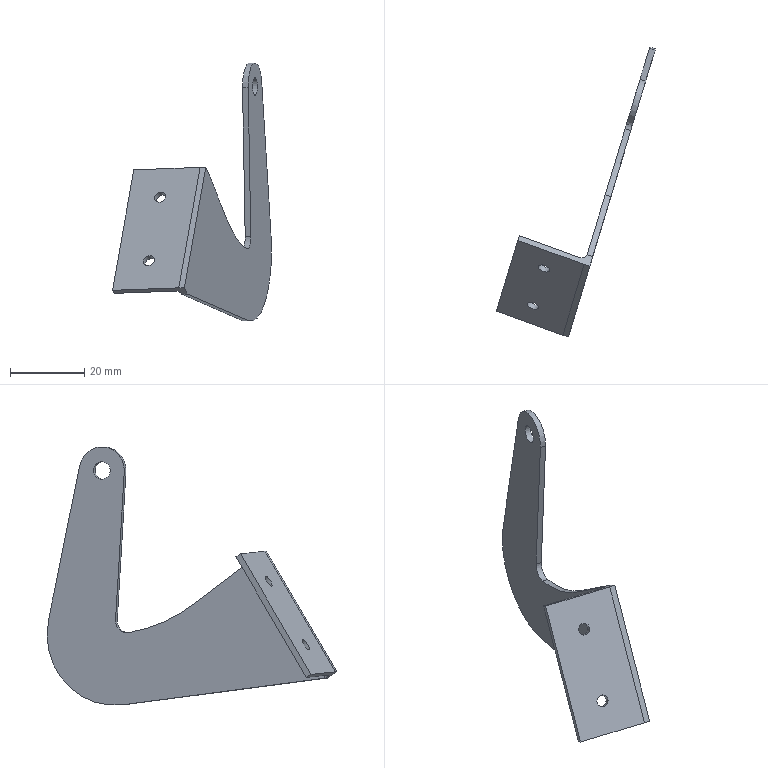Part | NX | features NG well(left door) 2 | 1 solid | 20 faces | box 42.889 x 78.177 x 69.7 mm | volume 5099 mm3 | plane 12 | cylinder 8 | commonest cylinder face diameters 3.175 x2 3.15 x1 4.763 x1 6.35 x1 12.7 x1 38.1 x1
STEP:
#1=CARTESIAN_POINT('',(72.317,-349.09,99.863));
#2=VERTEX_POINT('',#1);
#3=CARTESIAN_POINT('',(90.2,-355.62,100.522));
#4=VERTEX_POINT('',#3);
#5=CARTESIAN_POINT('',(90.2,-355.62,100.522));
#6=DIRECTION('',(0.9388,-0.3428,0.0346));
#7=VECTOR('',#6,1000.);
#8=LINE('',#5,#7);
#9=EDGE_CURVE('',#2,#4,#8,.T.);
#10=ORIENTED_EDGE('',*,*,#9,.T.);
#11=CARTESIAN_POINT('',(91.72,-356.079,100.522));
#12=VERTEX_POINT('',#11);
#13=CARTESIAN_POINT('',(90.2,-355.62,100.522));
#14=DIRECTION('',(0.9572,-0.2893,0.));
#15=VECTOR('',#14,1000.);
#16=LINE('',#13,#15);
#17=EDGE_CURVE('',#4,#12,#16,.T.);
#18=ORIENTED_EDGE('',*,*,#17,.T.);
#19=CARTESIAN_POINT('',(92.504,-353.486,98.866));
#20=VERTEX_POINT('',#19);
#21=CARTESIAN_POINT('',(91.72,-356.079,100.522));
#22=DIRECTION('',(-0.2468,-0.8167,0.5217));
#23=VECTOR('',#22,1000.);
#24=LINE('',#21,#23);
#25=EDGE_CURVE('',#20,#12,#24,.T.);
#26=ORIENTED_EDGE('',*,*,#25,.F.);
#27=CARTESIAN_POINT('',(90.982,-353.026,98.866));
#28=VERTEX_POINT('',#27);
#29=CARTESIAN_POINT('',(90.984,-353.027,98.866));
#30=DIRECTION('',(0.9572,-0.2893,0.));
#31=VECTOR('',#30,1000.);
#32=LINE('',#29,#31);
#33=EDGE_CURVE('',#28,#20,#32,.T.);
#34=ORIENTED_EDGE('',*,*,#33,.F.);
#35=CARTESIAN_POINT('',(89.01,-353.754,99.641));
#36=VERTEX_POINT('',#35);
#37=CARTESIAN_POINT('',(89.498,-352.501,98.821));
#38=DIRECTION('',(0.1509,0.4994,0.8531));
#39=DIRECTION('',(0.,-0.863,0.5052));
#40=AXIS2_PLACEMENT_3D('',#37,#38,#39);
#41=CIRCLE('',#40,1.575);
#42=EDGE_CURVE('',#28,#36,#41,.F.);
#43=ORIENTED_EDGE('',*,*,#42,.T.);
#44=CARTESIAN_POINT('',(72.805,-347.837,99.044));
#45=VERTEX_POINT('',#44);
#46=CARTESIAN_POINT('',(90.688,-354.367,99.703));
#47=DIRECTION('',(0.9388,-0.3428,0.0346));
#48=VECTOR('',#47,1000.);
#49=LINE('',#46,#48);
#50=EDGE_CURVE('',#45,#36,#49,.T.);
#51=ORIENTED_EDGE('',*,*,#50,.F.);
#52=CARTESIAN_POINT('',(72.805,-347.837,99.044));
#53=DIRECTION('',(-0.3097,-0.7957,0.5206));
#54=VECTOR('',#53,1000.);
#55=LINE('',#52,#54);
#56=EDGE_CURVE('',#45,#2,#55,.T.);
#57=ORIENTED_EDGE('',*,*,#56,.T.);
#58=EDGE_LOOP('',(#10,#18,#26,#34,#43,#51,#57));
#59=FACE_BOUND('',#58,.T.);
#60=CARTESIAN_POINT('',(90.2,-355.62,100.522));
#61=DIRECTION('',(0.1509,0.4994,0.8531));
#62=DIRECTION('',(0.,-0.863,0.5052));
#63=AXIS2_PLACEMENT_3D('',#60,#61,#62);
#64=PLANE('',#63);
#65=ADVANCED_FACE('',(#59),#64,.T.);
#66=CARTESIAN_POINT('',(97.419,-337.221,86.463));
#67=VERTEX_POINT('',#66);
#68=CARTESIAN_POINT('',(97.419,-337.221,86.463));
#69=DIRECTION('',(-0.2336,-0.7732,0.5896));
#70=VECTOR('',#69,1000.);
#71=LINE('',#68,#70);
#72=EDGE_CURVE('',#67,#20,#71,.T.);
#73=ORIENTED_EDGE('',*,*,#72,.F.);
#74=CARTESIAN_POINT('',(95.899,-336.762,86.463));
#75=VERTEX_POINT('',#74);
#76=CARTESIAN_POINT('',(95.899,-336.762,86.463));
#77=DIRECTION('',(0.9572,-0.2893,0.));
#78=VECTOR('',#77,1000.);
#79=LINE('',#76,#78);
#80=EDGE_CURVE('',#75,#67,#79,.T.);
#81=ORIENTED_EDGE('',*,*,#80,.F.);
#82=CARTESIAN_POINT('',(91.004,-352.96,98.815));
#83=VERTEX_POINT('',#82);
#84=CARTESIAN_POINT('',(95.899,-336.762,86.463));
#85=DIRECTION('',(-0.2336,-0.7732,0.5896));
#86=VECTOR('',#85,1000.);
#87=LINE('',#84,#86);
#88=EDGE_CURVE('',#75,#83,#87,.T.);
#89=ORIENTED_EDGE('',*,*,#88,.T.);
#90=CARTESIAN_POINT('',(89.497,-352.505,98.815));
#91=DIRECTION('',(0.1706,0.5644,0.8077));
#92=DIRECTION('',(-0.2336,-0.7732,0.5896));
#93=AXIS2_PLACEMENT_3D('',#90,#91,#92);
#94=ELLIPSE('',#93,1.58,1.575);
#95=EDGE_CURVE('',#83,#28,#94,.F.);
#96=ORIENTED_EDGE('',*,*,#95,.T.);
#97=ORIENTED_EDGE('',*,*,#33,.T.);
#98=EDGE_LOOP('',(#73,#81,#89,#96,#97));
#99=FACE_BOUND('',#98,.T.);
#100=CARTESIAN_POINT('',(95.899,-336.762,86.463));
#101=DIRECTION('',(0.1706,0.5644,0.8077));
#102=DIRECTION('',(0.,-0.8197,0.5728));
#103=AXIS2_PLACEMENT_3D('',#100,#101,#102);
#104=PLANE('',#103);
#105=ADVANCED_FACE('',(#99),#104,.T.);
#106=CARTESIAN_POINT('',(102.804,-319.401,78.568));
#107=VERTEX_POINT('',#106);
#108=CARTESIAN_POINT('',(105.,-312.134,122.365));
#109=DIRECTION('',(-0.9572,0.2893,0.));
#110=DIRECTION('',(0.2893,0.9572,0.));
#111=AXIS2_PLACEMENT_3D('',#108,#109,#110);
#112=CIRCLE('',#111,44.45);
#113=EDGE_CURVE('',#107,#67,#112,.T.);
#114=ORIENTED_EDGE('',*,*,#113,.F.);
#115=CARTESIAN_POINT('',(101.284,-318.942,78.568));
#116=VERTEX_POINT('',#115);
#117=CARTESIAN_POINT('',(101.284,-318.942,78.568));
#118=DIRECTION('',(0.9572,-0.2893,0.));
#119=VECTOR('',#118,1000.);
#120=LINE('',#117,#119);
#121=EDGE_CURVE('',#107,#116,#120,.F.);
#122=ORIENTED_EDGE('',*,*,#121,.T.);
#123=CARTESIAN_POINT('',(103.48,-311.675,122.365));
#124=DIRECTION('',(-0.9572,0.2893,0.));
#125=DIRECTION('',(0.2893,0.9572,0.));
#126=AXIS2_PLACEMENT_3D('',#123,#124,#125);
#127=CIRCLE('',#126,44.45);
#128=EDGE_CURVE('',#116,#75,#127,.T.);
#129=ORIENTED_EDGE('',*,*,#128,.T.);
#130=ORIENTED_EDGE('',*,*,#80,.T.);
#131=EDGE_LOOP('',(#114,#122,#129,#130));
#132=FACE_BOUND('',#131,.T.);
#133=CARTESIAN_POINT('',(103.48,-311.675,122.365));
#134=DIRECTION('',(0.9572,-0.2893,0.));
#135=DIRECTION('',(0.2893,0.9572,0.));
#136=AXIS2_PLACEMENT_3D('',#133,#134,#135);
#137=CYLINDRICAL_SURFACE('',#136,44.45);
#138=ADVANCED_FACE('',(#132),#137,.F.);
#139=CARTESIAN_POINT('',(101.647,-317.742,121.976));
#140=VERTEX_POINT('',#139);
#141=CARTESIAN_POINT('',(102.358,-315.389,81.891));
#142=VERTEX_POINT('',#141);
#143=CARTESIAN_POINT('',(101.647,-317.742,121.976));
#144=DIRECTION('',(0.0177,0.05858,-0.9981));
#145=VECTOR('',#144,1000.);
#146=LINE('',#143,#145);
#147=EDGE_CURVE('',#140,#142,#146,.T.);
#148=ORIENTED_EDGE('',*,*,#147,.T.);
#149=CARTESIAN_POINT('',(103.878,-315.849,81.891));
#150=VERTEX_POINT('',#149);
#151=CARTESIAN_POINT('',(103.878,-315.849,81.891));
#152=DIRECTION('',(-0.9572,0.2893,0.));
#153=VECTOR('',#152,1000.);
#154=LINE('',#151,#153);
#155=EDGE_CURVE('',#142,#150,#154,.F.);
#156=ORIENTED_EDGE('',*,*,#155,.T.);
#157=CARTESIAN_POINT('',(103.167,-318.201,121.976));
#158=VERTEX_POINT('',#157);
#159=CARTESIAN_POINT('',(103.167,-318.201,121.976));
#160=DIRECTION('',(0.0177,0.05858,-0.9981));
#161=VECTOR('',#160,1000.);
#162=LINE('',#159,#161);
#163=EDGE_CURVE('',#158,#150,#162,.T.);
#164=ORIENTED_EDGE('',*,*,#163,.F.);
#165=CARTESIAN_POINT('',(101.647,-317.742,121.976));
#166=DIRECTION('',(0.9572,-0.2893,0.));
#167=VECTOR('',#166,1000.);
#168=LINE('',#165,#167);
#169=EDGE_CURVE('',#140,#158,#168,.T.);
#170=ORIENTED_EDGE('',*,*,#169,.F.);
#171=EDGE_LOOP('',(#148,#156,#164,#170));
#172=FACE_BOUND('',#171,.T.);
#173=CARTESIAN_POINT('',(101.647,-317.742,121.976));
#174=DIRECTION('',(-0.2887,-0.9555,-0.0612));
#175=DIRECTION('',(0.9572,-0.2893,0.));
#176=AXIS2_PLACEMENT_3D('',#173,#174,#175);
#177=PLANE('',#176);
#178=ADVANCED_FACE('',(#172),#177,.T.);
#179=CARTESIAN_POINT('',(106.797,-306.186,123.674));
#180=VERTEX_POINT('',#179);
#181=CARTESIAN_POINT('',(105.,-312.134,122.365));
#182=DIRECTION('',(0.9572,-0.2893,0.));
#183=DIRECTION('',(0.2893,0.9572,0.));
#184=AXIS2_PLACEMENT_3D('',#181,#182,#183);
#185=CIRCLE('',#184,6.35);
#186=EDGE_CURVE('',#180,#158,#185,.T.);
#187=ORIENTED_EDGE('',*,*,#186,.F.);
#188=CARTESIAN_POINT('',(105.278,-305.727,123.674));
#189=VERTEX_POINT('',#188);
#190=CARTESIAN_POINT('',(105.278,-305.727,123.674));
#191=DIRECTION('',(0.9572,-0.2893,0.));
#192=VECTOR('',#191,1000.);
#193=LINE('',#190,#192);
#194=EDGE_CURVE('',#189,#180,#193,.T.);
#195=ORIENTED_EDGE('',*,*,#194,.F.);
#196=CARTESIAN_POINT('',(103.48,-311.675,122.365));
#197=DIRECTION('',(0.9572,-0.2893,0.));
#198=DIRECTION('',(0.2893,0.9572,0.));
#199=AXIS2_PLACEMENT_3D('',#196,#197,#198);
#200=CIRCLE('',#199,6.35);
#201=EDGE_CURVE('',#189,#140,#200,.T.);
#202=ORIENTED_EDGE('',*,*,#201,.T.);
#203=ORIENTED_EDGE('',*,*,#169,.T.);
#204=EDGE_LOOP('',(#187,#195,#202,#203));
#205=FACE_BOUND('',#204,.T.);
#206=CARTESIAN_POINT('',(103.48,-311.675,122.365));
#207=DIRECTION('',(0.9572,-0.2893,0.));
#208=DIRECTION('',(0.2893,0.9572,0.));
#209=AXIS2_PLACEMENT_3D('',#206,#207,#208);
#210=CYLINDRICAL_SURFACE('',#209,6.35);
#211=ADVANCED_FACE('',(#205),#210,.T.);
#212=CARTESIAN_POINT('',(109.338,-297.78,81.992));
#213=VERTEX_POINT('',#212);
#214=CARTESIAN_POINT('',(106.797,-306.186,123.674));
#215=DIRECTION('',(-0.05963,-0.1973,0.9785));
#216=VECTOR('',#215,1000.);
#217=LINE('',#214,#216);
#218=EDGE_CURVE('',#213,#180,#217,.T.);
#219=ORIENTED_EDGE('',*,*,#218,.F.);
#220=CARTESIAN_POINT('',(107.818,-297.321,81.992));
#221=VERTEX_POINT('',#220);
#222=CARTESIAN_POINT('',(107.818,-297.321,81.992));
#223=DIRECTION('',(0.9572,-0.2893,0.));
#224=VECTOR('',#223,1000.);
#225=LINE('',#222,#224);
#226=EDGE_CURVE('',#221,#213,#225,.T.);
#227=ORIENTED_EDGE('',*,*,#226,.F.);
#228=CARTESIAN_POINT('',(105.278,-305.727,123.674));
#229=DIRECTION('',(-0.05963,-0.1973,0.9785));
#230=VECTOR('',#229,1000.);
#231=LINE('',#228,#230);
#232=EDGE_CURVE('',#221,#189,#231,.T.);
#233=ORIENTED_EDGE('',*,*,#232,.T.);
#234=ORIENTED_EDGE('',*,*,#194,.T.);
#235=EDGE_LOOP('',(#219,#227,#233,#234));
#236=FACE_BOUND('',#235,.T.);
#237=CARTESIAN_POINT('',(105.278,-305.727,123.674));
#238=DIRECTION('',(0.2831,0.9367,0.2062));
#239=DIRECTION('',(-0.9572,0.2893,0.));
#240=AXIS2_PLACEMENT_3D('',#237,#238,#239);
#241=PLANE('',#240);
#242=ADVANCED_FACE('',(#236),#241,.T.);
#243=CARTESIAN_POINT('',(103.256,-317.907,59.165));
#244=VERTEX_POINT('',#243);
#245=CARTESIAN_POINT('',(103.945,-315.624,78.065));
#246=DIRECTION('',(0.9572,-0.2893,0.));
#247=DIRECTION('',(0.2893,0.9572,0.));
#248=AXIS2_PLACEMENT_3D('',#245,#246,#247);
#249=CIRCLE('',#248,19.05);
#250=EDGE_CURVE('',#244,#213,#249,.T.);
#251=ORIENTED_EDGE('',*,*,#250,.F.);
#252=CARTESIAN_POINT('',(101.736,-317.447,59.165));
#253=VERTEX_POINT('',#252);
#254=CARTESIAN_POINT('',(101.736,-317.447,59.165));
#255=DIRECTION('',(0.9572,-0.2893,0.));
#256=VECTOR('',#255,1000.);
#257=LINE('',#254,#256);
#258=EDGE_CURVE('',#253,#244,#257,.T.);
#259=ORIENTED_EDGE('',*,*,#258,.F.);
#260=CARTESIAN_POINT('',(102.426,-315.165,78.065));
#261=DIRECTION('',(0.9572,-0.2893,0.));
#262=DIRECTION('',(0.2893,0.9572,0.));
#263=AXIS2_PLACEMENT_3D('',#260,#261,#262);
#264=CIRCLE('',#263,19.05);
#265=EDGE_CURVE('',#253,#221,#264,.T.);
#266=ORIENTED_EDGE('',*,*,#265,.T.);
#267=ORIENTED_EDGE('',*,*,#226,.T.);
#268=EDGE_LOOP('',(#251,#259,#266,#267));
#269=FACE_BOUND('',#268,.T.);
#270=CARTESIAN_POINT('',(102.426,-315.165,78.065));
#271=DIRECTION('',(0.9572,-0.2893,0.));
#272=DIRECTION('',(0.2893,0.9572,0.));
#273=AXIS2_PLACEMENT_3D('',#270,#271,#272);
#274=CYLINDRICAL_SURFACE('',#273,19.05);
#275=ADVANCED_FACE('',(#269),#274,.T.);
#276=CARTESIAN_POINT('',(86.754,-372.514,66.362));
#277=VERTEX_POINT('',#276);
#278=CARTESIAN_POINT('',(86.754,-372.514,66.362));
#279=DIRECTION('',(0.287,0.9497,-0.1252));
#280=VECTOR('',#279,1000.);
#281=LINE('',#278,#280);
#282=EDGE_CURVE('',#277,#244,#281,.T.);
#283=ORIENTED_EDGE('',*,*,#282,.F.);
#284=CARTESIAN_POINT('',(85.232,-372.054,66.362));
#285=VERTEX_POINT('',#284);
#286=CARTESIAN_POINT('',(85.234,-372.054,66.362));
#287=DIRECTION('',(0.9572,-0.2893,0.));
#288=VECTOR('',#287,1000.);
#289=LINE('',#286,#288);
#290=EDGE_CURVE('',#285,#277,#289,.T.);
#291=ORIENTED_EDGE('',*,*,#290,.F.);
#292=CARTESIAN_POINT('',(85.261,-371.965,66.35));
#293=VERTEX_POINT('',#292);
#294=CARTESIAN_POINT('',(83.754,-371.509,66.35));
#295=DIRECTION('',(-0.03621,-0.1198,-0.9921));
#296=DIRECTION('',(0.287,0.9497,-0.1252));
#297=AXIS2_PLACEMENT_3D('',#294,#295,#296);
#298=ELLIPSE('',#297,1.727,1.575);
#299=EDGE_CURVE('',#285,#293,#298,.F.);
#300=ORIENTED_EDGE('',*,*,#299,.T.);
#301=CARTESIAN_POINT('',(85.234,-372.054,66.362));
#302=DIRECTION('',(0.287,0.9497,-0.1252));
#303=VECTOR('',#302,1000.);
#304=LINE('',#301,#303);
#305=EDGE_CURVE('',#293,#253,#304,.T.);
#306=ORIENTED_EDGE('',*,*,#305,.T.);
#307=ORIENTED_EDGE('',*,*,#258,.T.);
#308=EDGE_LOOP('',(#283,#291,#300,#306,#307));
#309=FACE_BOUND('',#308,.T.);
#310=CARTESIAN_POINT('',(85.234,-372.054,66.362));
#311=DIRECTION('',(-0.03621,-0.1198,-0.9921));
#312=DIRECTION('',(0.,0.9928,-0.1199));
#313=AXIS2_PLACEMENT_3D('',#310,#311,#312);
#314=PLANE('',#313);
#315=ADVANCED_FACE('',(#309),#314,.T.);
#316=CARTESIAN_POINT('',(84.451,-374.647,68.018));
#317=VERTEX_POINT('',#316);
#318=CARTESIAN_POINT('',(85.97,-375.106,68.018));
#319=VERTEX_POINT('',#318);
#320=CARTESIAN_POINT('',(84.451,-374.647,68.018));
#321=DIRECTION('',(0.9572,-0.2893,0.));
#322=VECTOR('',#321,1000.);
#323=LINE('',#320,#322);
#324=EDGE_CURVE('',#317,#319,#323,.T.);
#325=ORIENTED_EDGE('',*,*,#324,.F.);
#326=CARTESIAN_POINT('',(66.567,-368.117,67.359));
#327=VERTEX_POINT('',#326);
#328=CARTESIAN_POINT('',(84.451,-374.647,68.018));
#329=DIRECTION('',(-0.9388,0.3428,-0.0346));
#330=VECTOR('',#329,1000.);
#331=LINE('',#328,#330);
#332=EDGE_CURVE('',#317,#327,#331,.T.);
#333=ORIENTED_EDGE('',*,*,#332,.T.);
#334=CARTESIAN_POINT('',(67.055,-366.864,66.54));
#335=VERTEX_POINT('',#334);
#336=CARTESIAN_POINT('',(67.055,-366.864,66.54));
#337=DIRECTION('',(-0.3097,-0.7957,0.5206));
#338=VECTOR('',#337,1000.);
#339=LINE('',#336,#338);
#340=EDGE_CURVE('',#335,#327,#339,.T.);
#341=ORIENTED_EDGE('',*,*,#340,.F.);
#342=CARTESIAN_POINT('',(83.26,-372.781,67.137));
#343=VERTEX_POINT('',#342);
#344=CARTESIAN_POINT('',(84.938,-373.394,67.199));
#345=DIRECTION('',(-0.9388,0.3428,-0.0346));
#346=VECTOR('',#345,1000.);
#347=LINE('',#344,#346);
#348=EDGE_CURVE('',#343,#335,#347,.T.);
#349=ORIENTED_EDGE('',*,*,#348,.F.);
#350=CARTESIAN_POINT('',(83.748,-371.528,66.317));
#351=DIRECTION('',(-0.1509,-0.4994,-0.8531));
#352=DIRECTION('',(0.,0.863,-0.5052));
#353=AXIS2_PLACEMENT_3D('',#350,#351,#352);
#354=CIRCLE('',#353,1.575);
#355=EDGE_CURVE('',#343,#285,#354,.F.);
#356=ORIENTED_EDGE('',*,*,#355,.T.);
#357=ORIENTED_EDGE('',*,*,#290,.T.);
#358=CARTESIAN_POINT('',(86.754,-372.514,66.362));
#359=DIRECTION('',(0.2468,0.8167,-0.5217));
#360=VECTOR('',#359,1000.);
#361=LINE('',#358,#360);
#362=EDGE_CURVE('',#319,#277,#361,.T.);
#363=ORIENTED_EDGE('',*,*,#362,.F.);
#364=EDGE_LOOP('',(#325,#333,#341,#349,#356,#357,#363));
#365=FACE_BOUND('',#364,.T.);
#366=CARTESIAN_POINT('',(85.234,-372.054,66.362));
#367=DIRECTION('',(-0.1509,-0.4994,-0.8531));
#368=DIRECTION('',(0.,0.863,-0.5052));
#369=AXIS2_PLACEMENT_3D('',#366,#367,#368);
#370=PLANE('',#369);
#371=ADVANCED_FACE('',(#365),#370,.T.);
#372=CARTESIAN_POINT('',(91.72,-356.079,100.522));
#373=DIRECTION('',(-0.1509,-0.4994,-0.8531));
#374=VECTOR('',#373,1000.);
#375=LINE('',#372,#374);
#376=EDGE_CURVE('',#12,#319,#375,.T.);
#377=ORIENTED_EDGE('',*,*,#376,.F.);
#378=ORIENTED_EDGE('',*,*,#17,.F.);
#379=CARTESIAN_POINT('',(90.2,-355.62,100.522));
#380=DIRECTION('',(-0.1509,-0.4994,-0.8531));
#381=VECTOR('',#380,1000.);
#382=LINE('',#379,#381);
#383=EDGE_CURVE('',#4,#317,#382,.T.);
#384=ORIENTED_EDGE('',*,*,#383,.T.);
#385=ORIENTED_EDGE('',*,*,#324,.T.);
#386=EDGE_LOOP('',(#377,#378,#384,#385));
#387=FACE_BOUND('',#386,.T.);
#388=CARTESIAN_POINT('',(90.2,-355.62,100.522));
#389=DIRECTION('',(-0.2468,-0.8167,0.5217));
#390=DIRECTION('',(0.,-0.5384,-0.8427));
#391=AXIS2_PLACEMENT_3D('',#388,#389,#390);
#392=PLANE('',#391);
#393=ADVANCED_FACE('',(#387),#392,.T.);
#394=CARTESIAN_POINT('',(104.169,-309.396,122.365));
#395=VERTEX_POINT('',#394);
#396=CARTESIAN_POINT('',(103.48,-311.675,122.365));
#397=DIRECTION('',(0.9572,-0.2893,0.));
#398=DIRECTION('',(0.2893,0.9572,0.));
#399=AXIS2_PLACEMENT_3D('',#396,#397,#398);
#400=CIRCLE('',#399,2.381);
#401=EDGE_CURVE('',#395,#395,#400,.T.);
#402=ORIENTED_EDGE('',*,*,#401,.T.);
#403=EDGE_LOOP('',(#402));
#404=FACE_BOUND('',#403,.T.);
#405=ORIENTED_EDGE('',*,*,#305,.F.);
#406=CARTESIAN_POINT('',(97.432,-331.69,135.151));
#407=DIRECTION('',(0.1509,0.4994,0.8531));
#408=VECTOR('',#407,1000.);
#409=LINE('',#406,#408);
#410=EDGE_CURVE('',#293,#83,#409,.T.);
#411=ORIENTED_EDGE('',*,*,#410,.T.);
#412=ORIENTED_EDGE('',*,*,#88,.F.);
#413=ORIENTED_EDGE('',*,*,#128,.F.);
#414=CARTESIAN_POINT('',(101.441,-318.423,81.696));
#415=DIRECTION('',(0.9572,-0.2893,0.));
#416=DIRECTION('',(0.2893,0.9572,0.));
#417=AXIS2_PLACEMENT_3D('',#414,#415,#416);
#418=CIRCLE('',#417,3.175);
#419=EDGE_CURVE('',#116,#142,#418,.T.);
#420=ORIENTED_EDGE('',*,*,#419,.T.);
#421=ORIENTED_EDGE('',*,*,#147,.F.);
#422=ORIENTED_EDGE('',*,*,#201,.F.);
#423=ORIENTED_EDGE('',*,*,#232,.F.);
#424=ORIENTED_EDGE('',*,*,#265,.F.);
#425=EDGE_LOOP('',(#405,#411,#412,#413,#420,#421,#422,#423,#424));
#426=FACE_BOUND('',#425,.T.);
#427=CARTESIAN_POINT('',(103.48,-311.675,122.365));
#428=DIRECTION('',(0.9572,-0.2893,0.));
#429=DIRECTION('',(0.2893,0.9572,0.));
#430=AXIS2_PLACEMENT_3D('',#427,#428,#429);
#431=PLANE('',#430);
#432=ADVANCED_FACE('',(#404,#426),#431,.F.);
#433=CARTESIAN_POINT('',(105.689,-309.855,122.365));
#434=VERTEX_POINT('',#433);
#435=CARTESIAN_POINT('',(105.,-312.134,122.365));
#436=DIRECTION('',(0.9572,-0.2893,0.));
#437=DIRECTION('',(0.2893,0.9572,0.));
#438=AXIS2_PLACEMENT_3D('',#435,#436,#437);
#439=CIRCLE('',#438,2.381);
#440=EDGE_CURVE('',#434,#434,#439,.T.);
#441=ORIENTED_EDGE('',*,*,#440,.F.);
#442=EDGE_LOOP('',(#441));
#443=FACE_BOUND('',#442,.T.);
#444=ORIENTED_EDGE('',*,*,#25,.T.);
#445=ORIENTED_EDGE('',*,*,#376,.T.);
#446=ORIENTED_EDGE('',*,*,#362,.T.);
#447=ORIENTED_EDGE('',*,*,#282,.T.);
#448=ORIENTED_EDGE('',*,*,#250,.T.);
#449=ORIENTED_EDGE('',*,*,#218,.T.);
#450=ORIENTED_EDGE('',*,*,#186,.T.);
#451=ORIENTED_EDGE('',*,*,#163,.T.);
#452=CARTESIAN_POINT('',(102.961,-318.882,81.696));
#453=DIRECTION('',(0.9572,-0.2893,0.));
#454=DIRECTION('',(0.2893,0.9572,0.));
#455=AXIS2_PLACEMENT_3D('',#452,#453,#454);
#456=CIRCLE('',#455,3.175);
#457=EDGE_CURVE('',#150,#107,#456,.F.);
#458=ORIENTED_EDGE('',*,*,#457,.T.);
#459=ORIENTED_EDGE('',*,*,#113,.T.);
#460=ORIENTED_EDGE('',*,*,#72,.T.);
#461=EDGE_LOOP('',(#444,#445,#446,#447,#448,#449,#450,#451,#458,#459,#460));
#462=FACE_BOUND('',#461,.T.);
#463=CARTESIAN_POINT('',(105.,-312.134,122.365));
#464=DIRECTION('',(0.9572,-0.2893,0.));
#465=DIRECTION('',(0.2893,0.9572,0.));
#466=AXIS2_PLACEMENT_3D('',#463,#464,#465);
#467=PLANE('',#466);
#468=ADVANCED_FACE('',(#443,#462),#467,.T.);
#469=ORIENTED_EDGE('',*,*,#401,.F.);
#470=EDGE_LOOP('',(#469));
#471=FACE_BOUND('',#470,.T.);
#472=ORIENTED_EDGE('',*,*,#440,.T.);
#473=EDGE_LOOP('',(#472));
#474=FACE_BOUND('',#473,.T.);
#475=CARTESIAN_POINT('',(103.48,-311.675,122.365));
#476=DIRECTION('',(0.9572,-0.2893,0.));
#477=DIRECTION('',(0.2893,0.9572,0.));
#478=AXIS2_PLACEMENT_3D('',#475,#476,#477);
#479=CYLINDRICAL_SURFACE('',#478,2.381);
#480=ADVANCED_FACE('',(#471,#474),#479,.F.);
#481=ORIENTED_EDGE('',*,*,#419,.F.);
#482=ORIENTED_EDGE('',*,*,#121,.F.);
#483=ORIENTED_EDGE('',*,*,#457,.F.);
#484=ORIENTED_EDGE('',*,*,#155,.F.);
#485=EDGE_LOOP('',(#481,#482,#483,#484));
#486=FACE_BOUND('',#485,.T.);
#487=CARTESIAN_POINT('',(101.441,-318.423,81.696));
#488=DIRECTION('',(0.9572,-0.2893,0.));
#489=DIRECTION('',(0.2893,0.9572,0.));
#490=AXIS2_PLACEMENT_3D('',#487,#488,#489);
#491=CYLINDRICAL_SURFACE('',#490,3.175);
#492=ADVANCED_FACE('',(#486),#491,.F.);
#493=CARTESIAN_POINT('',(76.862,-366.324,73.201));
#494=VERTEX_POINT('',#493);
#495=CARTESIAN_POINT('',(76.862,-365.454,74.529));
#496=DIRECTION('',(-0.3097,-0.7957,0.5206));
#497=DIRECTION('',(0.,-0.5475,-0.8368));
#498=AXIS2_PLACEMENT_3D('',#495,#496,#497);
#499=CIRCLE('',#498,1.587);
#500=EDGE_CURVE('',#494,#494,#499,.T.);
#501=ORIENTED_EDGE('',*,*,#500,.T.);
#502=EDGE_LOOP('',(#501));
#503=FACE_BOUND('',#502,.T.);
#504=CARTESIAN_POINT('',(79.895,-356.286,90.348));
#505=VERTEX_POINT('',#504);
#506=CARTESIAN_POINT('',(79.895,-355.416,91.677));
#507=DIRECTION('',(-0.3097,-0.7957,0.5206));
#508=DIRECTION('',(0.,-0.5475,-0.8368));
#509=AXIS2_PLACEMENT_3D('',#506,#507,#508);
#510=CIRCLE('',#509,1.587);
#511=EDGE_CURVE('',#505,#505,#510,.T.);
#512=ORIENTED_EDGE('',*,*,#511,.T.);
#513=EDGE_LOOP('',(#512));
#514=FACE_BOUND('',#513,.T.);
#515=ORIENTED_EDGE('',*,*,#50,.T.);
#516=CARTESIAN_POINT('',(83.26,-372.781,67.137));
#517=DIRECTION('',(0.1509,0.4994,0.8531));
#518=VECTOR('',#517,1000.);
#519=LINE('',#516,#518);
#520=EDGE_CURVE('',#36,#343,#519,.F.);
#521=ORIENTED_EDGE('',*,*,#520,.T.);
#522=ORIENTED_EDGE('',*,*,#348,.T.);
#523=CARTESIAN_POINT('',(67.055,-366.864,66.54));
#524=DIRECTION('',(0.1509,0.4994,0.8531));
#525=VECTOR('',#524,1000.);
#526=LINE('',#523,#525);
#527=EDGE_CURVE('',#335,#45,#526,.T.);
#528=ORIENTED_EDGE('',*,*,#527,.T.);
#529=EDGE_LOOP('',(#515,#521,#522,#528));
#530=FACE_BOUND('',#529,.T.);
#531=CARTESIAN_POINT('',(84.938,-373.394,67.199));
#532=DIRECTION('',(0.3097,0.7957,-0.5206));
#533=DIRECTION('',(0.,0.5475,0.8368));
#534=AXIS2_PLACEMENT_3D('',#531,#532,#533);
#535=PLANE('',#534);
#536=ADVANCED_FACE('',(#503,#514,#530),#535,.T.);
#537=CARTESIAN_POINT('',(66.567,-368.117,67.359));
#538=DIRECTION('',(0.1509,0.4994,0.8531));
#539=VECTOR('',#538,1000.);
#540=LINE('',#537,#539);
#541=EDGE_CURVE('',#327,#2,#540,.T.);
#542=ORIENTED_EDGE('',*,*,#541,.T.);
#543=ORIENTED_EDGE('',*,*,#56,.F.);
#544=ORIENTED_EDGE('',*,*,#527,.F.);
#545=ORIENTED_EDGE('',*,*,#340,.T.);
#546=EDGE_LOOP('',(#542,#543,#544,#545));
#547=FACE_BOUND('',#546,.T.);
#548=CARTESIAN_POINT('',(67.055,-366.864,66.54));
#549=DIRECTION('',(0.9388,-0.3428,0.0346));
#550=DIRECTION('',(0.343,0.9393,0.));
#551=AXIS2_PLACEMENT_3D('',#548,#549,#550);
#552=PLANE('',#551);
#553=ADVANCED_FACE('',(#547),#552,.F.);
#554=CARTESIAN_POINT('',(76.374,-365.838,76.677));
#555=VERTEX_POINT('',#554);
#556=CARTESIAN_POINT('',(76.374,-366.707,75.349));
#557=DIRECTION('',(0.3097,0.7957,-0.5206));
#558=DIRECTION('',(0.,0.5475,0.8368));
#559=AXIS2_PLACEMENT_3D('',#556,#557,#558);
#560=CIRCLE('',#559,1.587);
#561=EDGE_CURVE('',#555,#555,#560,.T.);
#562=ORIENTED_EDGE('',*,*,#561,.T.);
#563=EDGE_LOOP('',(#562));
#564=FACE_BOUND('',#563,.T.);
#565=CARTESIAN_POINT('',(79.408,-355.8,93.825));
#566=VERTEX_POINT('',#565);
#567=CARTESIAN_POINT('',(79.408,-356.669,92.497));
#568=DIRECTION('',(0.3097,0.7957,-0.5206));
#569=DIRECTION('',(0.,0.5475,0.8368));
#570=AXIS2_PLACEMENT_3D('',#567,#568,#569);
#571=CIRCLE('',#570,1.587);
#572=EDGE_CURVE('',#566,#566,#571,.T.);
#573=ORIENTED_EDGE('',*,*,#572,.T.);
#574=EDGE_LOOP('',(#573));
#575=FACE_BOUND('',#574,.T.);
#576=ORIENTED_EDGE('',*,*,#383,.F.);
#577=ORIENTED_EDGE('',*,*,#9,.F.);
#578=ORIENTED_EDGE('',*,*,#541,.F.);
#579=ORIENTED_EDGE('',*,*,#332,.F.);
#580=EDGE_LOOP('',(#576,#577,#578,#579));
#581=FACE_BOUND('',#580,.T.);
#582=CARTESIAN_POINT('',(84.451,-374.647,68.018));
#583=DIRECTION('',(0.3097,0.7957,-0.5206));
#584=DIRECTION('',(0.,0.5475,0.8368));
#585=AXIS2_PLACEMENT_3D('',#582,#583,#584);
#586=PLANE('',#585);
#587=ADVANCED_FACE('',(#564,#575,#581),#586,.F.);
#588=ORIENTED_EDGE('',*,*,#355,.F.);
#589=ORIENTED_EDGE('',*,*,#520,.F.);
#590=ORIENTED_EDGE('',*,*,#42,.F.);
#591=ORIENTED_EDGE('',*,*,#95,.F.);
#592=ORIENTED_EDGE('',*,*,#410,.F.);
#593=ORIENTED_EDGE('',*,*,#299,.F.);
#594=EDGE_LOOP('',(#588,#589,#590,#591,#592,#593));
#595=FACE_BOUND('',#594,.T.);
#596=CARTESIAN_POINT('',(95.925,-331.234,135.151));
#597=DIRECTION('',(0.1509,0.4994,0.8531));
#598=DIRECTION('',(0.,-0.863,0.5052));
#599=AXIS2_PLACEMENT_3D('',#596,#597,#598);
#600=CYLINDRICAL_SURFACE('',#599,1.575);
#601=ADVANCED_FACE('',(#595),#600,.F.);
#602=ORIENTED_EDGE('',*,*,#511,.F.);
#603=EDGE_LOOP('',(#602));
#604=FACE_BOUND('',#603,.T.);
#605=ORIENTED_EDGE('',*,*,#572,.F.);
#606=EDGE_LOOP('',(#605));
#607=FACE_BOUND('',#606,.T.);
#608=CARTESIAN_POINT('',(79.895,-355.416,91.677));
#609=DIRECTION('',(-0.3097,-0.7957,0.5206));
#610=DIRECTION('',(0.,-0.5475,-0.8368));
#611=AXIS2_PLACEMENT_3D('',#608,#609,#610);
#612=CYLINDRICAL_SURFACE('',#611,1.587);
#613=ADVANCED_FACE('',(#604,#607),#612,.F.);
#614=ORIENTED_EDGE('',*,*,#500,.F.);
#615=EDGE_LOOP('',(#614));
#616=FACE_BOUND('',#615,.T.);
#617=ORIENTED_EDGE('',*,*,#561,.F.);
#618=EDGE_LOOP('',(#617));
#619=FACE_BOUND('',#618,.T.);
#620=CARTESIAN_POINT('',(76.862,-365.454,74.529));
#621=DIRECTION('',(-0.3097,-0.7957,0.5206));
#622=DIRECTION('',(0.,-0.5475,-0.8368));
#623=AXIS2_PLACEMENT_3D('',#620,#621,#622);
#624=CYLINDRICAL_SURFACE('',#623,1.587);
#625=ADVANCED_FACE('',(#616,#619),#624,.F.);
#626=CLOSED_SHELL('',(#65,#105,#138,#178,#211,#242,#275,#315,#371,#393,#432,#468,#480,#492,#536,#553,#587,#601,#613,#625));
#627=MANIFOLD_SOLID_BREP('',#626);
#628=(LENGTH_UNIT()NAMED_UNIT(*)SI_UNIT(.MILLI.,.METRE.));
#629=UNCERTAINTY_MEASURE_WITH_UNIT(LENGTH_MEASURE(0.00001),#628,'','');
#630=(NAMED_UNIT(*)PLANE_ANGLE_UNIT()SI_UNIT($,.RADIAN.));
#631=(NAMED_UNIT(*)SI_UNIT($,.STERADIAN.)SOLID_ANGLE_UNIT());
#632=(GEOMETRIC_REPRESENTATION_CONTEXT(3)GLOBAL_UNCERTAINTY_ASSIGNED_CONTEXT((#629))GLOBAL_UNIT_ASSIGNED_CONTEXT((#628,#630,#631))REPRESENTATION_CONTEXT('',''));
#633=ADVANCED_BREP_SHAPE_REPRESENTATION('',(#627),#632);